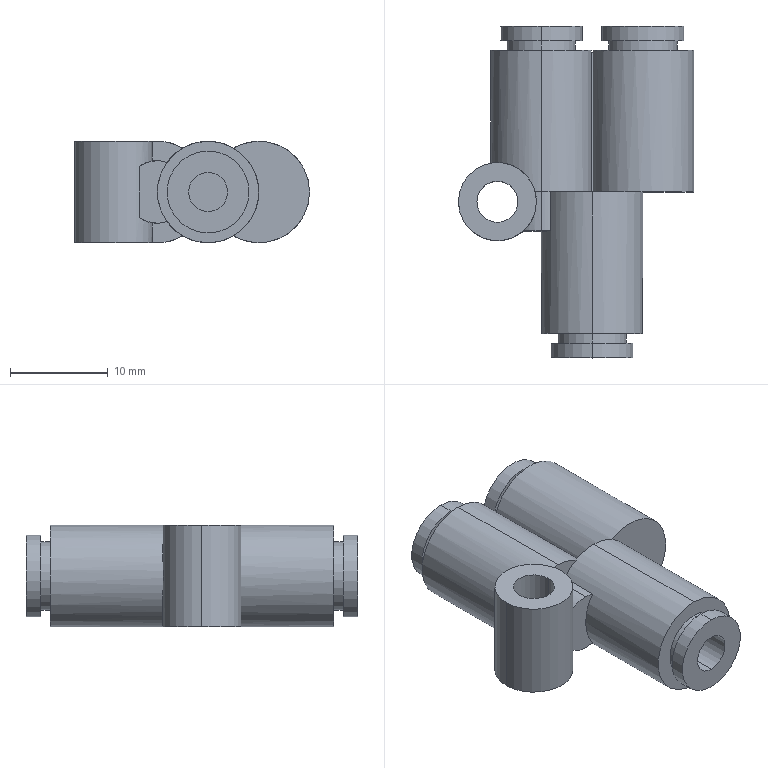Part | SolidWorks | features BaseBody 1 | 1 solid | 58 faces | box 24.1 x 34 x 10.4 mm | volume 3788 mm3 | cylinder 35 | plane 23 | commonest cylinder face diameters 10.4 x7 4 x6 7 x6 8.4 x6 2 x3 6.4 x3